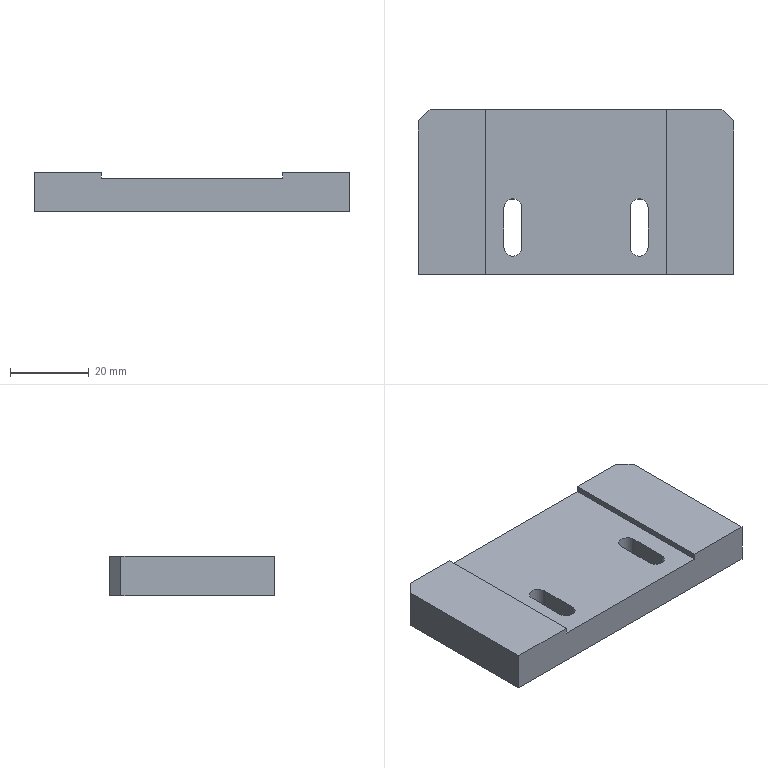Part | SolidWorks | features ICE 2, Chamfer 1, Extrusion 1, MirrorPattern 1 | 1 solid | 20 faces | box 80 x 42 x 10 mm | volume 29577 mm3 | plane 16 | cylinder 4 | commonest cylinder face diameters 4.5 x4
STEP:
#1=CARTESIAN_POINT('',(-18.25,-14.,0.));
#2=VERTEX_POINT('',#1);
#3=CARTESIAN_POINT('',(-13.75,-14.,0.));
#4=VERTEX_POINT('',#3);
#5=CARTESIAN_POINT('',(-16.,-14.,0.));
#6=DIRECTION('',(0.,0.,1.));
#7=DIRECTION('',(-1.,0.,0.));
#8=AXIS2_PLACEMENT_3D('',#5,#6,#7);
#9=CIRCLE('',#8,2.25);
#10=EDGE_CURVE('',#2,#4,#9,.T.);
#11=ORIENTED_EDGE('',*,*,#10,.T.);
#12=CARTESIAN_POINT('',(-13.75,-4.,0.));
#13=VERTEX_POINT('',#12);
#14=CARTESIAN_POINT('',(-13.75,-14.,0.));
#15=DIRECTION('',(0.,1.,0.));
#16=VECTOR('',#15,1000.);
#17=LINE('',#14,#16);
#18=EDGE_CURVE('',#4,#13,#17,.T.);
#19=ORIENTED_EDGE('',*,*,#18,.T.);
#20=CARTESIAN_POINT('',(-18.25,-4.,0.));
#21=VERTEX_POINT('',#20);
#22=CARTESIAN_POINT('',(-16.,-4.,0.));
#23=DIRECTION('',(0.,0.,1.));
#24=DIRECTION('',(-1.,0.,0.));
#25=AXIS2_PLACEMENT_3D('',#22,#23,#24);
#26=CIRCLE('',#25,2.25);
#27=EDGE_CURVE('',#13,#21,#26,.T.);
#28=ORIENTED_EDGE('',*,*,#27,.T.);
#29=CARTESIAN_POINT('',(-18.25,-14.,0.));
#30=DIRECTION('',(0.,-1.,0.));
#31=VECTOR('',#30,1000.);
#32=LINE('',#29,#31);
#33=EDGE_CURVE('',#21,#2,#32,.T.);
#34=ORIENTED_EDGE('',*,*,#33,.T.);
#35=EDGE_LOOP('',(#11,#19,#28,#34));
#36=FACE_BOUND('',#35,.T.);
#37=CARTESIAN_POINT('',(-40.,18.,0.));
#38=VERTEX_POINT('',#37);
#39=CARTESIAN_POINT('',(-40.,-21.,0.));
#40=VERTEX_POINT('',#39);
#41=CARTESIAN_POINT('',(-40.,-21.,0.));
#42=DIRECTION('',(0.,-1.,0.));
#43=VECTOR('',#42,1000.);
#44=LINE('',#41,#43);
#45=EDGE_CURVE('',#38,#40,#44,.T.);
#46=ORIENTED_EDGE('',*,*,#45,.F.);
#47=CARTESIAN_POINT('',(-37.,21.,0.));
#48=VERTEX_POINT('',#47);
#49=CARTESIAN_POINT('',(-29.,29.,0.));
#50=DIRECTION('',(0.7071,0.7071,0.));
#51=VECTOR('',#50,1000.);
#52=LINE('',#49,#51);
#53=EDGE_CURVE('',#38,#48,#52,.T.);
#54=ORIENTED_EDGE('',*,*,#53,.T.);
#55=CARTESIAN_POINT('',(37.,21.,0.));
#56=VERTEX_POINT('',#55);
#57=CARTESIAN_POINT('',(-40.,21.,0.));
#58=DIRECTION('',(-1.,0.,0.));
#59=VECTOR('',#58,1000.);
#60=LINE('',#57,#59);
#61=EDGE_CURVE('',#56,#48,#60,.T.);
#62=ORIENTED_EDGE('',*,*,#61,.F.);
#63=CARTESIAN_POINT('',(40.,18.,0.));
#64=VERTEX_POINT('',#63);
#65=CARTESIAN_POINT('',(29.,29.,0.));
#66=DIRECTION('',(0.7071,-0.7071,0.));
#67=VECTOR('',#66,1000.);
#68=LINE('',#65,#67);
#69=EDGE_CURVE('',#56,#64,#68,.T.);
#70=ORIENTED_EDGE('',*,*,#69,.T.);
#71=CARTESIAN_POINT('',(40.,-21.,0.));
#72=VERTEX_POINT('',#71);
#73=CARTESIAN_POINT('',(40.,-21.,0.));
#74=DIRECTION('',(0.,1.,0.));
#75=VECTOR('',#74,1000.);
#76=LINE('',#73,#75);
#77=EDGE_CURVE('',#72,#64,#76,.T.);
#78=ORIENTED_EDGE('',*,*,#77,.F.);
#79=CARTESIAN_POINT('',(-40.,-21.,0.));
#80=DIRECTION('',(1.,0.,0.));
#81=VECTOR('',#80,1000.);
#82=LINE('',#79,#81);
#83=EDGE_CURVE('',#40,#72,#82,.T.);
#84=ORIENTED_EDGE('',*,*,#83,.F.);
#85=EDGE_LOOP('',(#46,#54,#62,#70,#78,#84));
#86=FACE_OUTER_BOUND('',#85,.T.);
#87=CARTESIAN_POINT('',(13.75,-14.,0.));
#88=VERTEX_POINT('',#87);
#89=CARTESIAN_POINT('',(13.75,-4.,0.));
#90=VERTEX_POINT('',#89);
#91=CARTESIAN_POINT('',(13.75,-14.,0.));
#92=DIRECTION('',(0.,1.,0.));
#93=VECTOR('',#92,1000.);
#94=LINE('',#91,#93);
#95=EDGE_CURVE('',#88,#90,#94,.T.);
#96=ORIENTED_EDGE('',*,*,#95,.F.);
#97=CARTESIAN_POINT('',(18.25,-14.,0.));
#98=VERTEX_POINT('',#97);
#99=CARTESIAN_POINT('',(16.,-14.,0.));
#100=DIRECTION('',(0.,0.,-1.));
#101=DIRECTION('',(-1.,0.,0.));
#102=AXIS2_PLACEMENT_3D('',#99,#100,#101);
#103=CIRCLE('',#102,2.25);
#104=EDGE_CURVE('',#98,#88,#103,.T.);
#105=ORIENTED_EDGE('',*,*,#104,.F.);
#106=CARTESIAN_POINT('',(18.25,-4.,0.));
#107=VERTEX_POINT('',#106);
#108=CARTESIAN_POINT('',(18.25,-14.,0.));
#109=DIRECTION('',(0.,-1.,0.));
#110=VECTOR('',#109,1000.);
#111=LINE('',#108,#110);
#112=EDGE_CURVE('',#107,#98,#111,.T.);
#113=ORIENTED_EDGE('',*,*,#112,.F.);
#114=CARTESIAN_POINT('',(16.,-4.,0.));
#115=DIRECTION('',(0.,0.,-1.));
#116=DIRECTION('',(-1.,0.,0.));
#117=AXIS2_PLACEMENT_3D('',#114,#115,#116);
#118=CIRCLE('',#117,2.25);
#119=EDGE_CURVE('',#90,#107,#118,.T.);
#120=ORIENTED_EDGE('',*,*,#119,.F.);
#121=EDGE_LOOP('',(#96,#105,#113,#120));
#122=FACE_BOUND('',#121,.T.);
#123=CARTESIAN_POINT('',(0.,0.,0.));
#124=DIRECTION('',(0.,0.,-1.));
#125=DIRECTION('',(-1.,0.,0.));
#126=AXIS2_PLACEMENT_3D('',#123,#124,#125);
#127=PLANE('',#126);
#128=ADVANCED_FACE('',(#36,#86,#122),#127,.T.);
#129=CARTESIAN_POINT('',(23.,-21.,8.5));
#130=VERTEX_POINT('',#129);
#131=CARTESIAN_POINT('',(23.,21.,8.5));
#132=VERTEX_POINT('',#131);
#133=CARTESIAN_POINT('',(23.,-21.,8.5));
#134=DIRECTION('',(0.,1.,0.));
#135=VECTOR('',#134,1000.);
#136=LINE('',#133,#135);
#137=EDGE_CURVE('',#130,#132,#136,.T.);
#138=ORIENTED_EDGE('',*,*,#137,.T.);
#139=CARTESIAN_POINT('',(-23.,21.,8.5));
#140=VERTEX_POINT('',#139);
#141=CARTESIAN_POINT('',(-23.,21.,8.5));
#142=DIRECTION('',(-1.,0.,0.));
#143=VECTOR('',#142,1000.);
#144=LINE('',#141,#143);
#145=EDGE_CURVE('',#132,#140,#144,.T.);
#146=ORIENTED_EDGE('',*,*,#145,.T.);
#147=CARTESIAN_POINT('',(-23.,-21.,8.5));
#148=VERTEX_POINT('',#147);
#149=CARTESIAN_POINT('',(-23.,-21.,8.5));
#150=DIRECTION('',(0.,-1.,0.));
#151=VECTOR('',#150,1000.);
#152=LINE('',#149,#151);
#153=EDGE_CURVE('',#140,#148,#152,.T.);
#154=ORIENTED_EDGE('',*,*,#153,.T.);
#155=CARTESIAN_POINT('',(-23.,-21.,8.5));
#156=DIRECTION('',(1.,0.,0.));
#157=VECTOR('',#156,1000.);
#158=LINE('',#155,#157);
#159=EDGE_CURVE('',#148,#130,#158,.T.);
#160=ORIENTED_EDGE('',*,*,#159,.T.);
#161=EDGE_LOOP('',(#138,#146,#154,#160));
#162=FACE_OUTER_BOUND('',#161,.T.);
#163=CARTESIAN_POINT('',(-13.75,-14.,8.5));
#164=VERTEX_POINT('',#163);
#165=CARTESIAN_POINT('',(-13.75,-4.,8.5));
#166=VERTEX_POINT('',#165);
#167=CARTESIAN_POINT('',(-13.75,-14.,8.5));
#168=DIRECTION('',(0.,1.,0.));
#169=VECTOR('',#168,1000.);
#170=LINE('',#167,#169);
#171=EDGE_CURVE('',#164,#166,#170,.T.);
#172=ORIENTED_EDGE('',*,*,#171,.F.);
#173=CARTESIAN_POINT('',(-18.25,-14.,8.5));
#174=VERTEX_POINT('',#173);
#175=CARTESIAN_POINT('',(-16.,-14.,8.5));
#176=DIRECTION('',(0.,0.,1.));
#177=DIRECTION('',(1.,0.,0.));
#178=AXIS2_PLACEMENT_3D('',#175,#176,#177);
#179=CIRCLE('',#178,2.25);
#180=EDGE_CURVE('',#174,#164,#179,.T.);
#181=ORIENTED_EDGE('',*,*,#180,.F.);
#182=CARTESIAN_POINT('',(-18.25,-4.,8.5));
#183=VERTEX_POINT('',#182);
#184=CARTESIAN_POINT('',(-18.25,-14.,8.5));
#185=DIRECTION('',(0.,-1.,0.));
#186=VECTOR('',#185,1000.);
#187=LINE('',#184,#186);
#188=EDGE_CURVE('',#183,#174,#187,.T.);
#189=ORIENTED_EDGE('',*,*,#188,.F.);
#190=CARTESIAN_POINT('',(-16.,-4.,8.5));
#191=DIRECTION('',(0.,0.,1.));
#192=DIRECTION('',(1.,0.,0.));
#193=AXIS2_PLACEMENT_3D('',#190,#191,#192);
#194=CIRCLE('',#193,2.25);
#195=EDGE_CURVE('',#166,#183,#194,.T.);
#196=ORIENTED_EDGE('',*,*,#195,.F.);
#197=EDGE_LOOP('',(#172,#181,#189,#196));
#198=FACE_BOUND('',#197,.T.);
#199=CARTESIAN_POINT('',(18.25,-14.,8.5));
#200=VERTEX_POINT('',#199);
#201=CARTESIAN_POINT('',(13.75,-14.,8.5));
#202=VERTEX_POINT('',#201);
#203=CARTESIAN_POINT('',(16.,-14.,8.5));
#204=DIRECTION('',(0.,0.,-1.));
#205=DIRECTION('',(-1.,0.,0.));
#206=AXIS2_PLACEMENT_3D('',#203,#204,#205);
#207=CIRCLE('',#206,2.25);
#208=EDGE_CURVE('',#200,#202,#207,.T.);
#209=ORIENTED_EDGE('',*,*,#208,.T.);
#210=CARTESIAN_POINT('',(13.75,-4.,8.5));
#211=VERTEX_POINT('',#210);
#212=CARTESIAN_POINT('',(13.75,-14.,8.5));
#213=DIRECTION('',(0.,1.,0.));
#214=VECTOR('',#213,1000.);
#215=LINE('',#212,#214);
#216=EDGE_CURVE('',#202,#211,#215,.T.);
#217=ORIENTED_EDGE('',*,*,#216,.T.);
#218=CARTESIAN_POINT('',(18.25,-4.,8.5));
#219=VERTEX_POINT('',#218);
#220=CARTESIAN_POINT('',(16.,-4.,8.5));
#221=DIRECTION('',(0.,0.,-1.));
#222=DIRECTION('',(-1.,0.,0.));
#223=AXIS2_PLACEMENT_3D('',#220,#221,#222);
#224=CIRCLE('',#223,2.25);
#225=EDGE_CURVE('',#211,#219,#224,.T.);
#226=ORIENTED_EDGE('',*,*,#225,.T.);
#227=CARTESIAN_POINT('',(18.25,-14.,8.5));
#228=DIRECTION('',(0.,-1.,0.));
#229=VECTOR('',#228,1000.);
#230=LINE('',#227,#229);
#231=EDGE_CURVE('',#219,#200,#230,.T.);
#232=ORIENTED_EDGE('',*,*,#231,.T.);
#233=EDGE_LOOP('',(#209,#217,#226,#232));
#234=FACE_BOUND('',#233,.T.);
#235=CARTESIAN_POINT('',(0.,0.,8.5));
#236=DIRECTION('',(0.,0.,-1.));
#237=DIRECTION('',(-1.,0.,0.));
#238=AXIS2_PLACEMENT_3D('',#235,#236,#237);
#239=PLANE('',#238);
#240=ADVANCED_FACE('',(#162,#198,#234),#239,.F.);
#241=CARTESIAN_POINT('',(40.,-21.,10.));
#242=VERTEX_POINT('',#241);
#243=CARTESIAN_POINT('',(40.,18.,10.));
#244=VERTEX_POINT('',#243);
#245=CARTESIAN_POINT('',(40.,-21.,10.));
#246=DIRECTION('',(0.,1.,0.));
#247=VECTOR('',#246,1000.);
#248=LINE('',#245,#247);
#249=EDGE_CURVE('',#242,#244,#248,.T.);
#250=ORIENTED_EDGE('',*,*,#249,.T.);
#251=CARTESIAN_POINT('',(37.,21.,10.));
#252=VERTEX_POINT('',#251);
#253=CARTESIAN_POINT('',(37.,21.,10.));
#254=DIRECTION('',(-0.7071,0.7071,0.));
#255=VECTOR('',#254,1000.);
#256=LINE('',#253,#255);
#257=EDGE_CURVE('',#244,#252,#256,.T.);
#258=ORIENTED_EDGE('',*,*,#257,.T.);
#259=CARTESIAN_POINT('',(23.,21.,10.));
#260=VERTEX_POINT('',#259);
#261=CARTESIAN_POINT('',(-40.,21.,10.));
#262=DIRECTION('',(-1.,0.,0.));
#263=VECTOR('',#262,1000.);
#264=LINE('',#261,#263);
#265=EDGE_CURVE('',#252,#260,#264,.T.);
#266=ORIENTED_EDGE('',*,*,#265,.T.);
#267=CARTESIAN_POINT('',(23.,-21.,10.));
#268=VERTEX_POINT('',#267);
#269=CARTESIAN_POINT('',(23.,-21.,10.));
#270=DIRECTION('',(0.,1.,0.));
#271=VECTOR('',#270,1000.);
#272=LINE('',#269,#271);
#273=EDGE_CURVE('',#268,#260,#272,.T.);
#274=ORIENTED_EDGE('',*,*,#273,.F.);
#275=CARTESIAN_POINT('',(-40.,-21.,10.));
#276=DIRECTION('',(1.,0.,0.));
#277=VECTOR('',#276,1000.);
#278=LINE('',#275,#277);
#279=EDGE_CURVE('',#268,#242,#278,.T.);
#280=ORIENTED_EDGE('',*,*,#279,.T.);
#281=EDGE_LOOP('',(#250,#258,#266,#274,#280));
#282=FACE_OUTER_BOUND('',#281,.T.);
#283=CARTESIAN_POINT('',(0.,0.,10.));
#284=DIRECTION('',(0.,0.,-1.));
#285=DIRECTION('',(-1.,0.,0.));
#286=AXIS2_PLACEMENT_3D('',#283,#284,#285);
#287=PLANE('',#286);
#288=ADVANCED_FACE('',(#282),#287,.F.);
#289=ORIENTED_EDGE('',*,*,#77,.T.);
#290=CARTESIAN_POINT('',(40.,18.,10.));
#291=DIRECTION('',(0.,0.,1.));
#292=VECTOR('',#291,1000.);
#293=LINE('',#290,#292);
#294=EDGE_CURVE('',#64,#244,#293,.T.);
#295=ORIENTED_EDGE('',*,*,#294,.T.);
#296=ORIENTED_EDGE('',*,*,#249,.F.);
#297=CARTESIAN_POINT('',(40.,-21.,10.));
#298=DIRECTION('',(0.,0.,-1.));
#299=VECTOR('',#298,1000.);
#300=LINE('',#297,#299);
#301=EDGE_CURVE('',#242,#72,#300,.T.);
#302=ORIENTED_EDGE('',*,*,#301,.T.);
#303=EDGE_LOOP('',(#289,#295,#296,#302));
#304=FACE_OUTER_BOUND('',#303,.T.);
#305=CARTESIAN_POINT('',(40.,-21.,10.));
#306=DIRECTION('',(-1.,0.,0.));
#307=DIRECTION('',(0.,0.,1.));
#308=AXIS2_PLACEMENT_3D('',#305,#306,#307);
#309=PLANE('',#308);
#310=ADVANCED_FACE('',(#304),#309,.F.);
#311=ORIENTED_EDGE('',*,*,#61,.T.);
#312=CARTESIAN_POINT('',(-37.,21.,10.));
#313=VERTEX_POINT('',#312);
#314=CARTESIAN_POINT('',(-37.,21.,10.));
#315=DIRECTION('',(0.,0.,1.));
#316=VECTOR('',#315,1000.);
#317=LINE('',#314,#316);
#318=EDGE_CURVE('',#48,#313,#317,.T.);
#319=ORIENTED_EDGE('',*,*,#318,.T.);
#320=CARTESIAN_POINT('',(-23.,21.,10.));
#321=VERTEX_POINT('',#320);
#322=CARTESIAN_POINT('',(-40.,21.,10.));
#323=DIRECTION('',(-1.,0.,0.));
#324=VECTOR('',#323,1000.);
#325=LINE('',#322,#324);
#326=EDGE_CURVE('',#321,#313,#325,.T.);
#327=ORIENTED_EDGE('',*,*,#326,.F.);
#328=CARTESIAN_POINT('',(-23.,21.,8.5));
#329=DIRECTION('',(0.,0.,1.));
#330=VECTOR('',#329,1000.);
#331=LINE('',#328,#330);
#332=EDGE_CURVE('',#140,#321,#331,.T.);
#333=ORIENTED_EDGE('',*,*,#332,.F.);
#334=ORIENTED_EDGE('',*,*,#145,.F.);
#335=CARTESIAN_POINT('',(23.,21.,8.5));
#336=DIRECTION('',(0.,0.,1.));
#337=VECTOR('',#336,1000.);
#338=LINE('',#335,#337);
#339=EDGE_CURVE('',#132,#260,#338,.T.);
#340=ORIENTED_EDGE('',*,*,#339,.T.);
#341=ORIENTED_EDGE('',*,*,#265,.F.);
#342=CARTESIAN_POINT('',(37.,21.,10.));
#343=DIRECTION('',(0.,0.,-1.));
#344=VECTOR('',#343,1000.);
#345=LINE('',#342,#344);
#346=EDGE_CURVE('',#252,#56,#345,.T.);
#347=ORIENTED_EDGE('',*,*,#346,.T.);
#348=EDGE_LOOP('',(#311,#319,#327,#333,#334,#340,#341,#347));
#349=FACE_OUTER_BOUND('',#348,.T.);
#350=CARTESIAN_POINT('',(-40.,21.,10.));
#351=DIRECTION('',(0.,-1.,0.));
#352=DIRECTION('',(0.,0.,-1.));
#353=AXIS2_PLACEMENT_3D('',#350,#351,#352);
#354=PLANE('',#353);
#355=ADVANCED_FACE('',(#349),#354,.F.);
#356=CARTESIAN_POINT('',(-40.,18.,10.));
#357=VERTEX_POINT('',#356);
#358=CARTESIAN_POINT('',(-40.,-21.,10.));
#359=VERTEX_POINT('',#358);
#360=CARTESIAN_POINT('',(-40.,-21.,10.));
#361=DIRECTION('',(0.,-1.,0.));
#362=VECTOR('',#361,1000.);
#363=LINE('',#360,#362);
#364=EDGE_CURVE('',#357,#359,#363,.T.);
#365=ORIENTED_EDGE('',*,*,#364,.F.);
#366=CARTESIAN_POINT('',(-40.,18.,10.));
#367=DIRECTION('',(0.,0.,-1.));
#368=VECTOR('',#367,1000.);
#369=LINE('',#366,#368);
#370=EDGE_CURVE('',#357,#38,#369,.T.);
#371=ORIENTED_EDGE('',*,*,#370,.T.);
#372=ORIENTED_EDGE('',*,*,#45,.T.);
#373=CARTESIAN_POINT('',(-40.,-21.,10.));
#374=DIRECTION('',(0.,0.,-1.));
#375=VECTOR('',#374,1000.);
#376=LINE('',#373,#375);
#377=EDGE_CURVE('',#359,#40,#376,.T.);
#378=ORIENTED_EDGE('',*,*,#377,.F.);
#379=EDGE_LOOP('',(#365,#371,#372,#378));
#380=FACE_OUTER_BOUND('',#379,.T.);
#381=CARTESIAN_POINT('',(-40.,-21.,10.));
#382=DIRECTION('',(1.,0.,0.));
#383=DIRECTION('',(0.,0.,-1.));
#384=AXIS2_PLACEMENT_3D('',#381,#382,#383);
#385=PLANE('',#384);
#386=ADVANCED_FACE('',(#380),#385,.F.);
#387=ORIENTED_EDGE('',*,*,#279,.F.);
#388=CARTESIAN_POINT('',(23.,-21.,8.5));
#389=DIRECTION('',(0.,0.,1.));
#390=VECTOR('',#389,1000.);
#391=LINE('',#388,#390);
#392=EDGE_CURVE('',#130,#268,#391,.T.);
#393=ORIENTED_EDGE('',*,*,#392,.F.);
#394=ORIENTED_EDGE('',*,*,#159,.F.);
#395=CARTESIAN_POINT('',(-23.,-21.,10.));
#396=VERTEX_POINT('',#395);
#397=CARTESIAN_POINT('',(-23.,-21.,8.5));
#398=DIRECTION('',(0.,0.,1.));
#399=VECTOR('',#398,1000.);
#400=LINE('',#397,#399);
#401=EDGE_CURVE('',#148,#396,#400,.T.);
#402=ORIENTED_EDGE('',*,*,#401,.T.);
#403=CARTESIAN_POINT('',(-40.,-21.,10.));
#404=DIRECTION('',(1.,0.,0.));
#405=VECTOR('',#404,1000.);
#406=LINE('',#403,#405);
#407=EDGE_CURVE('',#359,#396,#406,.T.);
#408=ORIENTED_EDGE('',*,*,#407,.F.);
#409=ORIENTED_EDGE('',*,*,#377,.T.);
#410=ORIENTED_EDGE('',*,*,#83,.T.);
#411=ORIENTED_EDGE('',*,*,#301,.F.);
#412=EDGE_LOOP('',(#387,#393,#394,#402,#408,#409,#410,#411));
#413=FACE_OUTER_BOUND('',#412,.T.);
#414=CARTESIAN_POINT('',(-40.,-21.,10.));
#415=DIRECTION('',(0.,1.,0.));
#416=DIRECTION('',(0.,0.,1.));
#417=AXIS2_PLACEMENT_3D('',#414,#415,#416);
#418=PLANE('',#417);
#419=ADVANCED_FACE('',(#413),#418,.F.);
#420=ORIENTED_EDGE('',*,*,#326,.T.);
#421=CARTESIAN_POINT('',(-40.,18.,10.));
#422=DIRECTION('',(-0.7071,-0.7071,0.));
#423=VECTOR('',#422,1000.);
#424=LINE('',#421,#423);
#425=EDGE_CURVE('',#313,#357,#424,.T.);
#426=ORIENTED_EDGE('',*,*,#425,.T.);
#427=ORIENTED_EDGE('',*,*,#364,.T.);
#428=ORIENTED_EDGE('',*,*,#407,.T.);
#429=CARTESIAN_POINT('',(-23.,-21.,10.));
#430=DIRECTION('',(0.,-1.,0.));
#431=VECTOR('',#430,1000.);
#432=LINE('',#429,#431);
#433=EDGE_CURVE('',#321,#396,#432,.T.);
#434=ORIENTED_EDGE('',*,*,#433,.F.);
#435=EDGE_LOOP('',(#420,#426,#427,#428,#434));
#436=FACE_OUTER_BOUND('',#435,.T.);
#437=CARTESIAN_POINT('',(0.,0.,10.));
#438=DIRECTION('',(0.,0.,-1.));
#439=DIRECTION('',(-1.,0.,0.));
#440=AXIS2_PLACEMENT_3D('',#437,#438,#439);
#441=PLANE('',#440);
#442=ADVANCED_FACE('',(#436),#441,.F.);
#443=ORIENTED_EDGE('',*,*,#273,.T.);
#444=ORIENTED_EDGE('',*,*,#339,.F.);
#445=ORIENTED_EDGE('',*,*,#137,.F.);
#446=ORIENTED_EDGE('',*,*,#392,.T.);
#447=EDGE_LOOP('',(#443,#444,#445,#446));
#448=FACE_OUTER_BOUND('',#447,.T.);
#449=CARTESIAN_POINT('',(23.,-21.,8.5));
#450=DIRECTION('',(1.,0.,0.));
#451=DIRECTION('',(0.,0.,-1.));
#452=AXIS2_PLACEMENT_3D('',#449,#450,#451);
#453=PLANE('',#452);
#454=ADVANCED_FACE('',(#448),#453,.F.);
#455=ORIENTED_EDGE('',*,*,#433,.T.);
#456=ORIENTED_EDGE('',*,*,#401,.F.);
#457=ORIENTED_EDGE('',*,*,#153,.F.);
#458=ORIENTED_EDGE('',*,*,#332,.T.);
#459=EDGE_LOOP('',(#455,#456,#457,#458));
#460=FACE_OUTER_BOUND('',#459,.T.);
#461=CARTESIAN_POINT('',(-23.,-21.,8.5));
#462=DIRECTION('',(-1.,0.,0.));
#463=DIRECTION('',(0.,0.,1.));
#464=AXIS2_PLACEMENT_3D('',#461,#462,#463);
#465=PLANE('',#464);
#466=ADVANCED_FACE('',(#460),#465,.F.);
#467=ORIENTED_EDGE('',*,*,#425,.F.);
#468=ORIENTED_EDGE('',*,*,#318,.F.);
#469=ORIENTED_EDGE('',*,*,#53,.F.);
#470=ORIENTED_EDGE('',*,*,#370,.F.);
#471=EDGE_LOOP('',(#467,#468,#469,#470));
#472=FACE_OUTER_BOUND('',#471,.T.);
#473=CARTESIAN_POINT('',(-40.,18.,10.));
#474=DIRECTION('',(0.7071,-0.7071,0.));
#475=DIRECTION('',(0.,0.,-1.));
#476=AXIS2_PLACEMENT_3D('',#473,#474,#475);
#477=PLANE('',#476);
#478=ADVANCED_FACE('',(#472),#477,.F.);
#479=ORIENTED_EDGE('',*,*,#257,.F.);
#480=ORIENTED_EDGE('',*,*,#294,.F.);
#481=ORIENTED_EDGE('',*,*,#69,.F.);
#482=ORIENTED_EDGE('',*,*,#346,.F.);
#483=EDGE_LOOP('',(#479,#480,#481,#482));
#484=FACE_OUTER_BOUND('',#483,.T.);
#485=CARTESIAN_POINT('',(37.,21.,10.));
#486=DIRECTION('',(-0.7071,-0.7071,0.));
#487=DIRECTION('',(0.,0.,-1.));
#488=AXIS2_PLACEMENT_3D('',#485,#486,#487);
#489=PLANE('',#488);
#490=ADVANCED_FACE('',(#484),#489,.F.);
#491=CARTESIAN_POINT('',(-18.25,-14.,-0.001));
#492=DIRECTION('',(0.,0.,1.));
#493=VECTOR('',#492,1000.);
#494=LINE('',#491,#493);
#495=EDGE_CURVE('',#2,#174,#494,.T.);
#496=ORIENTED_EDGE('',*,*,#495,.T.);
#497=ORIENTED_EDGE('',*,*,#180,.T.);
#498=CARTESIAN_POINT('',(-13.75,-14.,-0.001));
#499=DIRECTION('',(0.,0.,1.));
#500=VECTOR('',#499,1000.);
#501=LINE('',#498,#500);
#502=EDGE_CURVE('',#4,#164,#501,.T.);
#503=ORIENTED_EDGE('',*,*,#502,.F.);
#504=ORIENTED_EDGE('',*,*,#10,.F.);
#505=EDGE_LOOP('',(#496,#497,#503,#504));
#506=FACE_OUTER_BOUND('',#505,.T.);
#507=CARTESIAN_POINT('',(-16.,-14.,-0.001));
#508=DIRECTION('',(0.,0.,1.));
#509=DIRECTION('',(1.,0.,0.));
#510=AXIS2_PLACEMENT_3D('',#507,#508,#509);
#511=CYLINDRICAL_SURFACE('',#510,2.25);
#512=ADVANCED_FACE('',(#506),#511,.F.);
#513=CARTESIAN_POINT('',(-18.25,-4.,-0.001));
#514=DIRECTION('',(0.,0.,1.));
#515=VECTOR('',#514,1000.);
#516=LINE('',#513,#515);
#517=EDGE_CURVE('',#21,#183,#516,.T.);
#518=ORIENTED_EDGE('',*,*,#517,.T.);
#519=ORIENTED_EDGE('',*,*,#188,.T.);
#520=ORIENTED_EDGE('',*,*,#495,.F.);
#521=ORIENTED_EDGE('',*,*,#33,.F.);
#522=EDGE_LOOP('',(#518,#519,#520,#521));
#523=FACE_OUTER_BOUND('',#522,.T.);
#524=CARTESIAN_POINT('',(-18.25,-14.,-0.001));
#525=DIRECTION('',(-1.,0.,0.));
#526=DIRECTION('',(0.,-1.,0.));
#527=AXIS2_PLACEMENT_3D('',#524,#525,#526);
#528=PLANE('',#527);
#529=ADVANCED_FACE('',(#523),#528,.F.);
#530=CARTESIAN_POINT('',(-13.75,-4.,-0.001));
#531=DIRECTION('',(0.,0.,1.));
#532=VECTOR('',#531,1000.);
#533=LINE('',#530,#532);
#534=EDGE_CURVE('',#13,#166,#533,.T.);
#535=ORIENTED_EDGE('',*,*,#534,.T.);
#536=ORIENTED_EDGE('',*,*,#195,.T.);
#537=ORIENTED_EDGE('',*,*,#517,.F.);
#538=ORIENTED_EDGE('',*,*,#27,.F.);
#539=EDGE_LOOP('',(#535,#536,#537,#538));
#540=FACE_OUTER_BOUND('',#539,.T.);
#541=CARTESIAN_POINT('',(-16.,-4.,-0.001));
#542=DIRECTION('',(0.,0.,1.));
#543=DIRECTION('',(1.,0.,0.));
#544=AXIS2_PLACEMENT_3D('',#541,#542,#543);
#545=CYLINDRICAL_SURFACE('',#544,2.25);
#546=ADVANCED_FACE('',(#540),#545,.F.);
#547=ORIENTED_EDGE('',*,*,#502,.T.);
#548=ORIENTED_EDGE('',*,*,#171,.T.);
#549=ORIENTED_EDGE('',*,*,#534,.F.);
#550=ORIENTED_EDGE('',*,*,#18,.F.);
#551=EDGE_LOOP('',(#547,#548,#549,#550));
#552=FACE_OUTER_BOUND('',#551,.T.);
#553=CARTESIAN_POINT('',(-13.75,-14.,-0.001));
#554=DIRECTION('',(1.,0.,0.));
#555=DIRECTION('',(0.,1.,0.));
#556=AXIS2_PLACEMENT_3D('',#553,#554,#555);
#557=PLANE('',#556);
#558=ADVANCED_FACE('',(#552),#557,.F.);
#559=ORIENTED_EDGE('',*,*,#104,.T.);
#560=CARTESIAN_POINT('',(13.75,-14.,-0.001));
#561=DIRECTION('',(0.,0.,1.));
#562=VECTOR('',#561,1000.);
#563=LINE('',#560,#562);
#564=EDGE_CURVE('',#88,#202,#563,.T.);
#565=ORIENTED_EDGE('',*,*,#564,.T.);
#566=ORIENTED_EDGE('',*,*,#208,.F.);
#567=CARTESIAN_POINT('',(18.25,-14.,-0.001));
#568=DIRECTION('',(0.,0.,1.));
#569=VECTOR('',#568,1000.);
#570=LINE('',#567,#569);
#571=EDGE_CURVE('',#98,#200,#570,.T.);
#572=ORIENTED_EDGE('',*,*,#571,.F.);
#573=EDGE_LOOP('',(#559,#565,#566,#572));
#574=FACE_OUTER_BOUND('',#573,.T.);
#575=CARTESIAN_POINT('',(16.,-14.,-0.001));
#576=DIRECTION('',(0.,0.,1.));
#577=DIRECTION('',(1.,0.,0.));
#578=AXIS2_PLACEMENT_3D('',#575,#576,#577);
#579=CYLINDRICAL_SURFACE('',#578,2.25);
#580=ADVANCED_FACE('',(#574),#579,.F.);
#581=ORIENTED_EDGE('',*,*,#95,.T.);
#582=CARTESIAN_POINT('',(13.75,-4.,-0.001));
#583=DIRECTION('',(0.,0.,1.));
#584=VECTOR('',#583,1000.);
#585=LINE('',#582,#584);
#586=EDGE_CURVE('',#90,#211,#585,.T.);
#587=ORIENTED_EDGE('',*,*,#586,.T.);
#588=ORIENTED_EDGE('',*,*,#216,.F.);
#589=ORIENTED_EDGE('',*,*,#564,.F.);
#590=EDGE_LOOP('',(#581,#587,#588,#589));
#591=FACE_OUTER_BOUND('',#590,.T.);
#592=CARTESIAN_POINT('',(13.75,-14.,-0.001));
#593=DIRECTION('',(1.,0.,0.));
#594=DIRECTION('',(0.,1.,0.));
#595=AXIS2_PLACEMENT_3D('',#592,#593,#594);
#596=PLANE('',#595);
#597=ADVANCED_FACE('',(#591),#596,.T.);
#598=ORIENTED_EDGE('',*,*,#119,.T.);
#599=CARTESIAN_POINT('',(18.25,-4.,-0.001));
#600=DIRECTION('',(0.,0.,1.));
#601=VECTOR('',#600,1000.);
#602=LINE('',#599,#601);
#603=EDGE_CURVE('',#107,#219,#602,.T.);
#604=ORIENTED_EDGE('',*,*,#603,.T.);
#605=ORIENTED_EDGE('',*,*,#225,.F.);
#606=ORIENTED_EDGE('',*,*,#586,.F.);
#607=EDGE_LOOP('',(#598,#604,#605,#606));
#608=FACE_OUTER_BOUND('',#607,.T.);
#609=CARTESIAN_POINT('',(16.,-4.,-0.001));
#610=DIRECTION('',(0.,0.,1.));
#611=DIRECTION('',(1.,0.,0.));
#612=AXIS2_PLACEMENT_3D('',#609,#610,#611);
#613=CYLINDRICAL_SURFACE('',#612,2.25);
#614=ADVANCED_FACE('',(#608),#613,.F.);
#615=ORIENTED_EDGE('',*,*,#112,.T.);
#616=ORIENTED_EDGE('',*,*,#571,.T.);
#617=ORIENTED_EDGE('',*,*,#231,.F.);
#618=ORIENTED_EDGE('',*,*,#603,.F.);
#619=EDGE_LOOP('',(#615,#616,#617,#618));
#620=FACE_OUTER_BOUND('',#619,.T.);
#621=CARTESIAN_POINT('',(18.25,-14.,-0.001));
#622=DIRECTION('',(-1.,0.,0.));
#623=DIRECTION('',(0.,-1.,0.));
#624=AXIS2_PLACEMENT_3D('',#621,#622,#623);
#625=PLANE('',#624);
#626=ADVANCED_FACE('',(#620),#625,.T.);
#627=CLOSED_SHELL('',(#128,#240,#288,#310,#355,#386,#419,#442,#454,#466,#478,#490,#512,#529,#546,#558,#580,#597,#614,#626));
#628=MANIFOLD_SOLID_BREP('',#627);
#629=CARTESIAN_POINT('',(0.,0.,0.));
#630=DIRECTION('',(0.,0.,1.));
#631=DIRECTION('',(1.,0.,0.));
#632=AXIS2_PLACEMENT_3D('',#629,#630,#631);
#633=(LENGTH_UNIT()NAMED_UNIT(*)SI_UNIT(.MILLI.,.METRE.));
#634=UNCERTAINTY_MEASURE_WITH_UNIT(LENGTH_MEASURE(0.00001),#633,'','');
#635=(NAMED_UNIT(*)PLANE_ANGLE_UNIT()SI_UNIT($,.RADIAN.));
#636=(NAMED_UNIT(*)SI_UNIT($,.STERADIAN.)SOLID_ANGLE_UNIT());
#637=(GEOMETRIC_REPRESENTATION_CONTEXT(3)GLOBAL_UNCERTAINTY_ASSIGNED_CONTEXT((#634))GLOBAL_UNIT_ASSIGNED_CONTEXT((#633,#635,#636))REPRESENTATION_CONTEXT('',''));
#638=ADVANCED_BREP_SHAPE_REPRESENTATION('',(#628,#632),#637);